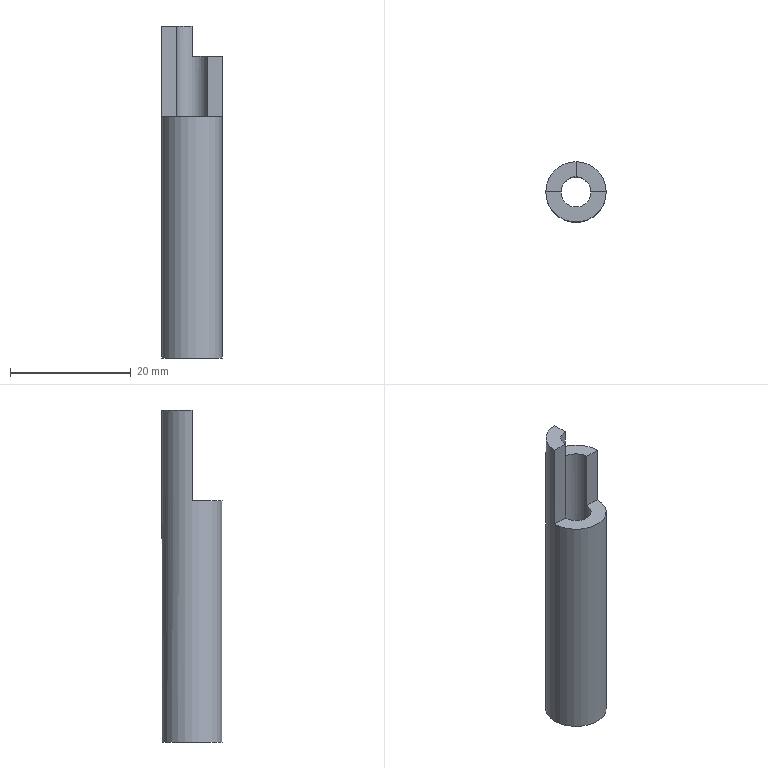Part | STEP file | SWF10-15_id1854_x_t | 1 solid | 9 faces | box 10 x 10 x 55 mm | volume 2723 mm3 | plane 7 | cylinder 2 | commonest cylinder face diameters 5.003 x1 10 x1
STEP:
#1=CARTESIAN_POINT('',(339.498,-22.5,-85.));
#2=VERTEX_POINT('',#1);
#3=CARTESIAN_POINT('',(342.,-22.5,-85.));
#4=DIRECTION('',(0.,0.,1.));
#5=DIRECTION('',(-1.,0.,0.));
#6=AXIS2_PLACEMENT_3D('',#3,#4,#5);
#7=CIRCLE('',#6,2.502);
#8=EDGE_CURVE('',#2,#2,#7,.T.);
#9=ORIENTED_EDGE('',*,*,#8,.T.);
#10=EDGE_LOOP('',(#9));
#11=FACE_BOUND('',#10,.T.);
#12=CARTESIAN_POINT('',(337.,-22.5,-85.));
#13=VERTEX_POINT('',#12);
#14=CARTESIAN_POINT('',(342.,-22.5,-85.));
#15=DIRECTION('',(0.,0.,1.));
#16=DIRECTION('',(-1.,0.,0.));
#17=AXIS2_PLACEMENT_3D('',#14,#15,#16);
#18=CIRCLE('',#17,5.);
#19=EDGE_CURVE('',#13,#13,#18,.T.);
#20=ORIENTED_EDGE('',*,*,#19,.F.);
#21=EDGE_LOOP('',(#20));
#22=FACE_BOUND('',#21,.T.);
#23=CARTESIAN_POINT('',(342.,-22.5,-85.));
#24=DIRECTION('',(0.,0.,-1.));
#25=DIRECTION('',(-1.,0.,0.));
#26=AXIS2_PLACEMENT_3D('',#23,#24,#25);
#27=PLANE('',#26);
#28=ADVANCED_FACE('',(#11,#22),#27,.T.);
#29=CARTESIAN_POINT('',(342.,-17.5,-30.));
#30=VERTEX_POINT('',#29);
#31=CARTESIAN_POINT('',(342.,-19.998,-30.));
#32=VERTEX_POINT('',#31);
#33=CARTESIAN_POINT('',(342.,-22.5,-30.));
#34=DIRECTION('',(0.,-1.,0.));
#35=VECTOR('',#34,1.);
#36=LINE('',#33,#35);
#37=EDGE_CURVE('',#30,#32,#36,.T.);
#38=ORIENTED_EDGE('',*,*,#37,.F.);
#39=CARTESIAN_POINT('',(337.,-22.5,-30.));
#40=VERTEX_POINT('',#39);
#41=CARTESIAN_POINT('',(342.,-22.5,-30.));
#42=DIRECTION('',(0.,0.,-1.));
#43=DIRECTION('',(1.,0.,0.));
#44=AXIS2_PLACEMENT_3D('',#41,#42,#43);
#45=CIRCLE('',#44,5.);
#46=EDGE_CURVE('',#40,#30,#45,.T.);
#47=ORIENTED_EDGE('',*,*,#46,.F.);
#48=CARTESIAN_POINT('',(339.498,-22.5,-30.));
#49=VERTEX_POINT('',#48);
#50=CARTESIAN_POINT('',(342.,-22.5,-30.));
#51=DIRECTION('',(1.,0.,0.));
#52=VECTOR('',#51,1.);
#53=LINE('',#50,#52);
#54=EDGE_CURVE('',#40,#49,#53,.T.);
#55=ORIENTED_EDGE('',*,*,#54,.T.);
#56=CARTESIAN_POINT('',(342.,-22.5,-30.));
#57=DIRECTION('',(0.,0.,-1.));
#58=DIRECTION('',(1.,0.,0.));
#59=AXIS2_PLACEMENT_3D('',#56,#57,#58);
#60=CIRCLE('',#59,2.502);
#61=EDGE_CURVE('',#49,#32,#60,.T.);
#62=ORIENTED_EDGE('',*,*,#61,.T.);
#63=EDGE_LOOP('',(#38,#47,#55,#62));
#64=FACE_OUTER_BOUND('',#63,.T.);
#65=CARTESIAN_POINT('',(342.,-22.5,-30.));
#66=DIRECTION('',(0.,0.,1.));
#67=DIRECTION('',(1.,0.,0.));
#68=AXIS2_PLACEMENT_3D('',#65,#66,#67);
#69=PLANE('',#68);
#70=ADVANCED_FACE('',(#64),#69,.T.);
#71=CARTESIAN_POINT('',(342.,-17.5,-35.));
#72=VERTEX_POINT('',#71);
#73=CARTESIAN_POINT('',(342.,-17.5,-2.));
#74=DIRECTION('',(0.,0.,1.));
#75=VECTOR('',#74,1.);
#76=LINE('',#73,#75);
#77=EDGE_CURVE('',#72,#30,#76,.T.);
#78=ORIENTED_EDGE('',*,*,#77,.F.);
#79=CARTESIAN_POINT('',(347.,-22.5,-35.));
#80=VERTEX_POINT('',#79);
#81=CARTESIAN_POINT('',(342.,-22.5,-35.));
#82=DIRECTION('',(0.,0.,-1.));
#83=DIRECTION('',(1.,0.,0.));
#84=AXIS2_PLACEMENT_3D('',#81,#82,#83);
#85=CIRCLE('',#84,5.);
#86=EDGE_CURVE('',#72,#80,#85,.T.);
#87=ORIENTED_EDGE('',*,*,#86,.T.);
#88=CARTESIAN_POINT('',(347.,-22.5,-45.));
#89=VERTEX_POINT('',#88);
#90=CARTESIAN_POINT('',(347.,-22.5,-2.));
#91=DIRECTION('',(0.,0.,-1.));
#92=VECTOR('',#91,1.);
#93=LINE('',#90,#92);
#94=EDGE_CURVE('',#80,#89,#93,.T.);
#95=ORIENTED_EDGE('',*,*,#94,.T.);
#96=CARTESIAN_POINT('',(337.,-22.5,-45.));
#97=VERTEX_POINT('',#96);
#98=CARTESIAN_POINT('',(342.,-22.5,-45.));
#99=DIRECTION('',(0.,0.,-1.));
#100=DIRECTION('',(1.,0.,0.));
#101=AXIS2_PLACEMENT_3D('',#98,#99,#100);
#102=CIRCLE('',#101,5.);
#103=EDGE_CURVE('',#89,#97,#102,.T.);
#104=ORIENTED_EDGE('',*,*,#103,.T.);
#105=CARTESIAN_POINT('',(337.,-22.5,-2.));
#106=DIRECTION('',(0.,0.,1.));
#107=VECTOR('',#106,1.);
#108=LINE('',#105,#107);
#109=EDGE_CURVE('',#97,#40,#108,.T.);
#110=ORIENTED_EDGE('',*,*,#109,.T.);
#111=ORIENTED_EDGE('',*,*,#46,.T.);
#112=EDGE_LOOP('',(#78,#87,#95,#104,#110,#111));
#113=FACE_BOUND('',#112,.T.);
#114=ORIENTED_EDGE('',*,*,#19,.T.);
#115=EDGE_LOOP('',(#114));
#116=FACE_BOUND('',#115,.T.);
#117=CARTESIAN_POINT('',(342.,-22.5,-2.));
#118=DIRECTION('',(0.,0.,-1.));
#119=DIRECTION('',(-1.,0.,0.));
#120=AXIS2_PLACEMENT_3D('',#117,#118,#119);
#121=CYLINDRICAL_SURFACE('',#120,5.);
#122=ADVANCED_FACE('',(#113,#116),#121,.T.);
#123=CARTESIAN_POINT('',(342.,-19.998,-35.));
#124=VERTEX_POINT('',#123);
#125=CARTESIAN_POINT('',(344.502,-22.5,-35.));
#126=VERTEX_POINT('',#125);
#127=CARTESIAN_POINT('',(342.,-22.5,-35.));
#128=DIRECTION('',(0.,0.,-1.));
#129=DIRECTION('',(1.,0.,0.));
#130=AXIS2_PLACEMENT_3D('',#127,#128,#129);
#131=CIRCLE('',#130,2.502);
#132=EDGE_CURVE('',#124,#126,#131,.T.);
#133=ORIENTED_EDGE('',*,*,#132,.F.);
#134=CARTESIAN_POINT('',(342.,-19.998,-2.));
#135=DIRECTION('',(0.,0.,1.));
#136=VECTOR('',#135,1.);
#137=LINE('',#134,#136);
#138=EDGE_CURVE('',#124,#32,#137,.T.);
#139=ORIENTED_EDGE('',*,*,#138,.T.);
#140=ORIENTED_EDGE('',*,*,#61,.F.);
#141=CARTESIAN_POINT('',(339.498,-22.5,-45.));
#142=VERTEX_POINT('',#141);
#143=CARTESIAN_POINT('',(339.498,-22.5,-2.));
#144=DIRECTION('',(0.,0.,1.));
#145=VECTOR('',#144,1.);
#146=LINE('',#143,#145);
#147=EDGE_CURVE('',#142,#49,#146,.T.);
#148=ORIENTED_EDGE('',*,*,#147,.F.);
#149=CARTESIAN_POINT('',(344.502,-22.5,-45.));
#150=VERTEX_POINT('',#149);
#151=CARTESIAN_POINT('',(342.,-22.5,-45.));
#152=DIRECTION('',(0.,0.,-1.));
#153=DIRECTION('',(1.,0.,0.));
#154=AXIS2_PLACEMENT_3D('',#151,#152,#153);
#155=CIRCLE('',#154,2.502);
#156=EDGE_CURVE('',#150,#142,#155,.T.);
#157=ORIENTED_EDGE('',*,*,#156,.F.);
#158=CARTESIAN_POINT('',(344.502,-22.5,-2.));
#159=DIRECTION('',(0.,0.,-1.));
#160=VECTOR('',#159,1.);
#161=LINE('',#158,#160);
#162=EDGE_CURVE('',#126,#150,#161,.T.);
#163=ORIENTED_EDGE('',*,*,#162,.F.);
#164=EDGE_LOOP('',(#133,#139,#140,#148,#157,#163));
#165=FACE_BOUND('',#164,.T.);
#166=ORIENTED_EDGE('',*,*,#8,.F.);
#167=EDGE_LOOP('',(#166));
#168=FACE_BOUND('',#167,.T.);
#169=CARTESIAN_POINT('',(342.,-22.5,-2.));
#170=DIRECTION('',(0.,0.,-1.));
#171=DIRECTION('',(-1.,0.,0.));
#172=AXIS2_PLACEMENT_3D('',#169,#170,#171);
#173=CYLINDRICAL_SURFACE('',#172,2.502);
#174=ADVANCED_FACE('',(#165,#168),#173,.F.);
#175=CARTESIAN_POINT('',(342.,-22.5,-35.));
#176=DIRECTION('',(0.,-1.,0.));
#177=VECTOR('',#176,1.);
#178=LINE('',#175,#177);
#179=EDGE_CURVE('',#72,#124,#178,.T.);
#180=ORIENTED_EDGE('',*,*,#179,.T.);
#181=ORIENTED_EDGE('',*,*,#132,.T.);
#182=CARTESIAN_POINT('',(367.,-22.5,-35.));
#183=DIRECTION('',(1.,0.,0.));
#184=VECTOR('',#183,1.);
#185=LINE('',#182,#184);
#186=EDGE_CURVE('',#126,#80,#185,.T.);
#187=ORIENTED_EDGE('',*,*,#186,.T.);
#188=ORIENTED_EDGE('',*,*,#86,.F.);
#189=EDGE_LOOP('',(#180,#181,#187,#188));
#190=FACE_OUTER_BOUND('',#189,.T.);
#191=CARTESIAN_POINT('',(367.,2.5,-35.));
#192=DIRECTION('',(0.,0.,1.));
#193=DIRECTION('',(1.,0.,0.));
#194=AXIS2_PLACEMENT_3D('',#191,#192,#193);
#195=PLANE('',#194);
#196=ADVANCED_FACE('',(#190),#195,.T.);
#197=ORIENTED_EDGE('',*,*,#186,.F.);
#198=ORIENTED_EDGE('',*,*,#162,.T.);
#199=CARTESIAN_POINT('',(342.,-22.5,-45.));
#200=DIRECTION('',(1.,0.,0.));
#201=VECTOR('',#200,1.);
#202=LINE('',#199,#201);
#203=EDGE_CURVE('',#150,#89,#202,.T.);
#204=ORIENTED_EDGE('',*,*,#203,.T.);
#205=ORIENTED_EDGE('',*,*,#94,.F.);
#206=EDGE_LOOP('',(#197,#198,#204,#205));
#207=FACE_OUTER_BOUND('',#206,.T.);
#208=CARTESIAN_POINT('',(342.,-22.5,-17.));
#209=DIRECTION('',(0.,-1.,0.));
#210=DIRECTION('',(0.,0.,-1.));
#211=AXIS2_PLACEMENT_3D('',#208,#209,#210);
#212=PLANE('',#211);
#213=ADVANCED_FACE('',(#207),#212,.T.);
#214=ORIENTED_EDGE('',*,*,#203,.F.);
#215=ORIENTED_EDGE('',*,*,#156,.T.);
#216=CARTESIAN_POINT('',(342.,-22.5,-45.));
#217=DIRECTION('',(1.,0.,0.));
#218=VECTOR('',#217,1.);
#219=LINE('',#216,#218);
#220=EDGE_CURVE('',#97,#142,#219,.T.);
#221=ORIENTED_EDGE('',*,*,#220,.F.);
#222=ORIENTED_EDGE('',*,*,#103,.F.);
#223=EDGE_LOOP('',(#214,#215,#221,#222));
#224=FACE_OUTER_BOUND('',#223,.T.);
#225=CARTESIAN_POINT('',(367.,2.5,-45.));
#226=DIRECTION('',(0.,0.,1.));
#227=DIRECTION('',(1.,0.,0.));
#228=AXIS2_PLACEMENT_3D('',#225,#226,#227);
#229=PLANE('',#228);
#230=ADVANCED_FACE('',(#224),#229,.T.);
#231=ORIENTED_EDGE('',*,*,#77,.T.);
#232=ORIENTED_EDGE('',*,*,#37,.T.);
#233=ORIENTED_EDGE('',*,*,#138,.F.);
#234=ORIENTED_EDGE('',*,*,#179,.F.);
#235=EDGE_LOOP('',(#231,#232,#233,#234));
#236=FACE_OUTER_BOUND('',#235,.T.);
#237=CARTESIAN_POINT('',(342.,-22.5,90.));
#238=DIRECTION('',(-1.,0.,0.));
#239=DIRECTION('',(0.,0.,-1.));
#240=AXIS2_PLACEMENT_3D('',#237,#238,#239);
#241=PLANE('',#240);
#242=ADVANCED_FACE('',(#236),#241,.F.);
#243=ORIENTED_EDGE('',*,*,#220,.T.);
#244=ORIENTED_EDGE('',*,*,#147,.T.);
#245=ORIENTED_EDGE('',*,*,#54,.F.);
#246=ORIENTED_EDGE('',*,*,#109,.F.);
#247=EDGE_LOOP('',(#243,#244,#245,#246));
#248=FACE_OUTER_BOUND('',#247,.T.);
#249=CARTESIAN_POINT('',(342.,-22.5,-17.));
#250=DIRECTION('',(0.,-1.,0.));
#251=DIRECTION('',(0.,0.,-1.));
#252=AXIS2_PLACEMENT_3D('',#249,#250,#251);
#253=PLANE('',#252);
#254=ADVANCED_FACE('',(#248),#253,.T.);
#255=CLOSED_SHELL('',(#28,#70,#122,#174,#196,#213,#230,#242,#254));
#256=MANIFOLD_SOLID_BREP('',#255);
#257=(LENGTH_UNIT()NAMED_UNIT(*)SI_UNIT(.MILLI.,.METRE.));
#258=UNCERTAINTY_MEASURE_WITH_UNIT(LENGTH_MEASURE(0.00002),#257,'','');
#259=(NAMED_UNIT(*)PLANE_ANGLE_UNIT()SI_UNIT($,.RADIAN.));
#260=PLANE_ANGLE_MEASURE_WITH_UNIT(PLANE_ANGLE_MEASURE(0.01745),#259);
#261=DIMENSIONAL_EXPONENTS(0.,0.,0.,0.,0.,0.,0.);
#262=(CONVERSION_BASED_UNIT('DEGREE',#260)NAMED_UNIT(#261)PLANE_ANGLE_UNIT());
#263=(NAMED_UNIT(*)SI_UNIT($,.STERADIAN.)SOLID_ANGLE_UNIT());
#264=(GEOMETRIC_REPRESENTATION_CONTEXT(3)GLOBAL_UNCERTAINTY_ASSIGNED_CONTEXT((#258))GLOBAL_UNIT_ASSIGNED_CONTEXT((#257,#262,#263))REPRESENTATION_CONTEXT('',''));
#265=ADVANCED_BREP_SHAPE_REPRESENTATION('',(#256),#264);